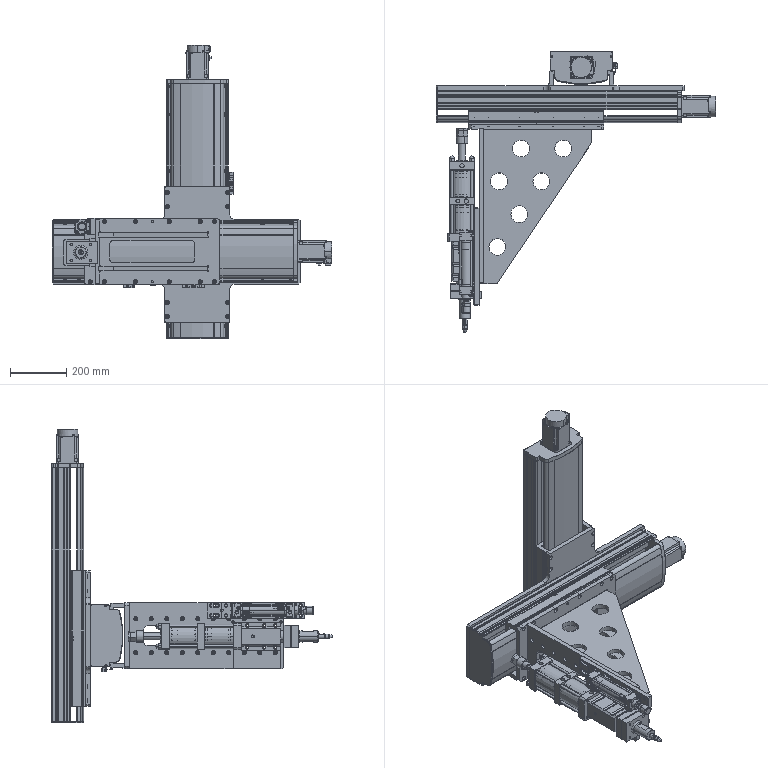Part | SolidWorks | features ReferencePattern 3, CompositeCurve 2, LocalLPattern 1 | 112 solids | 4971 faces | volume 39439593 mm3 | cylinder 2278 | plane 2093 | cone 420 | torus 126 | spline 54 | commonest cylinder face diameters 15 x284 6.8 x170 8.6 x168 9 x163 5.5 x88 6 x76